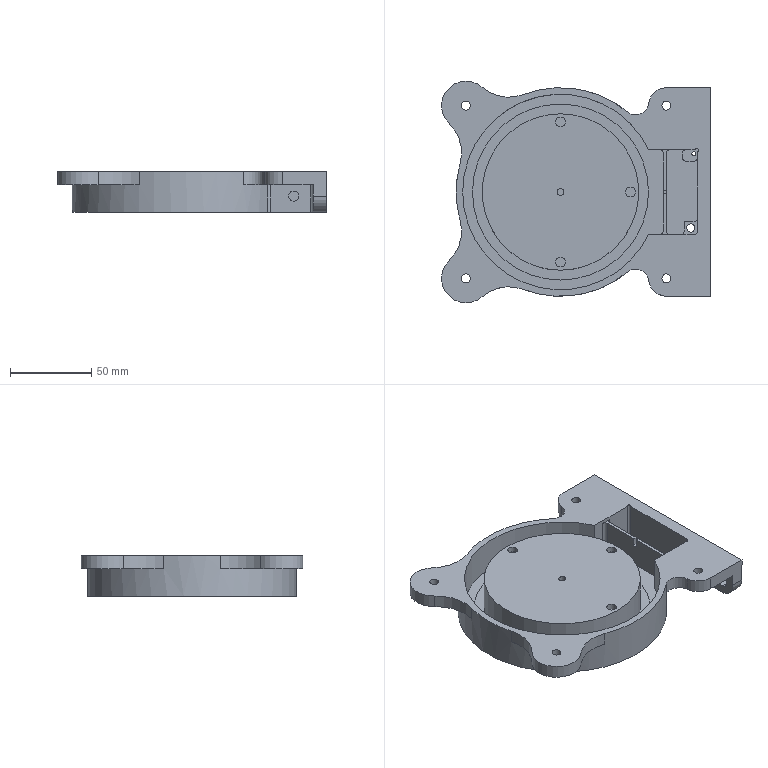NC program | NX | posted with a generic post | part box 165 x 136 x 25 mm
Lines 3306 to 5148 of 5148, first 1627 of 1827 lines:
(CAVITY_MILL_COPY_COPY , TOOL : D4)
N6580 T04 M6
N6582 G54
N6584 G17 G0 G90 X13.936 Y-32.8 S9500 M3
N6586 G43 Z30. H4
N6588 Z0.605
N6590 G94 G1 Z-0.395 F1000.
N6592 X13.763 Y-32.5
N6594 G3 X12.897 Y-32. R1.
N6596 G1 X10. F1500.
N6598 Y-34.897
N6600 G3 X10.5 Y-35.763 R1.
N6602 G1 X10.8 Y-35.936
N6604 Z0.605
N6606 G0 Z30.
N6608 X13.936 Y-32.8
N6610 Z0.209
N6612 G1 Z-0.791 F1000.
N6614 X13.763 Y-32.5
N6616 G3 X12.897 Y-32. R1.
N6618 G1 X10. F1500.
N6620 Y-34.897
N6622 G3 X10.5 Y-35.763 R1.
N6624 G1 X10.8 Y-35.936
N6626 Z0.209
N6628 G0 X13.936 Y-32.8 Z-0.186
N6630 G1 Z-1.186 F1000.
N6632 X13.763 Y-32.5
N6634 G3 X12.897 Y-32. R1.
N6636 G1 X10. F1500.
N6638 Y-34.897
N6640 G3 X10.5 Y-35.763 R1.
N6642 G1 X10.8 Y-35.936
N6644 Z-0.186
N6646 G0 X13.936 Y-32.8 Z-0.581
N6648 G1 Z-1.581 F1000.
N6650 X13.763 Y-32.5
N6652 G3 X12.897 Y-32. R1.
N6654 G1 X10. F1500.
N6656 Y-34.897
N6658 G3 X10.5 Y-35.763 R1.
N6660 G1 X10.8 Y-35.936
N6662 Z-0.581
N6664 G0 X13.936 Y-32.8 Z-0.977
N6666 G1 Z-1.977 F1000.
N6668 X13.763 Y-32.5
N6670 G3 X12.897 Y-32. R1.
N6672 G1 X10. F1500.
N6674 Y-34.897
N6676 G3 X10.5 Y-35.763 R1.
N6678 G1 X10.8 Y-35.936
N6680 Z-0.977
N6682 G0 X13.936 Y-32.8 Z-1.372
N6684 G1 Z-2.372 F1000.
N6686 X13.763 Y-32.5
N6688 G3 X12.897 Y-32. R1.
N6690 G1 X10. F1500.
N6692 Y-34.897
N6694 G3 X10.5 Y-35.763 R1.
N6696 G1 X10.8 Y-35.936
N6698 Z-1.372
N6700 G0 X13.936 Y-32.8 Z-1.767
N6702 G1 Z-2.767 F1000.
N6704 X13.763 Y-32.5
N6706 G3 X12.897 Y-32. R1.
N6708 G1 X10. F1500.
N6710 Y-34.897
N6712 G3 X10.5 Y-35.763 R1.
N6714 G1 X10.8 Y-35.936
N6716 Z-1.767
N6718 G0 X13.936 Y-32.8 Z-2.163
N6720 G1 Z-3.163 F1000.
N6722 X13.763 Y-32.5
N6724 G3 X12.897 Y-32. R1.
N6726 G1 X10. F1500.
N6728 Y-34.897
N6730 G3 X10.5 Y-35.763 R1.
N6732 G1 X10.8 Y-35.936
N6734 Z-2.163
N6736 G0 X13.936 Y-32.8 Z-2.558
N6738 G1 Z-3.558 F1000.
N6740 X13.763 Y-32.5
N6742 G3 X12.897 Y-32. R1.
N6744 G1 X10. F1500.
N6746 Y-34.897
N6748 G3 X10.5 Y-35.763 R1.
N6750 G1 X10.8 Y-35.936
N6752 Z-2.558
N6754 G0 X13.936 Y-32.8 Z-2.953
N6756 G1 Z-3.953 F1000.
N6758 X13.763 Y-32.5
N6760 G3 X12.897 Y-32. R1.
N6762 G1 X10. F1500.
N6764 Y-34.897
N6766 G3 X10.5 Y-35.763 R1.
N6768 G1 X10.8 Y-35.936
N6770 Z-2.953
N6772 G0 X13.936 Y-32.8 Z-3.349
N6774 G1 Z-4.349 F1000.
N6776 X13.763 Y-32.5
N6778 G3 X12.897 Y-32. R1.
N6780 G1 X10. F1500.
N6782 Y-34.897
N6784 G3 X10.5 Y-35.763 R1.
N6786 G1 X10.8 Y-35.936
N6788 Z-3.349
N6790 G0 X13.936 Y-32.8 Z-3.744
N6792 G1 Z-4.744 F1000.
N6794 X13.763 Y-32.5
N6796 G3 X12.897 Y-32. R1.
N6798 G1 X10. F1500.
N6800 Y-34.897
N6802 G3 X10.5 Y-35.763 R1.
N6804 G1 X10.8 Y-35.936
N6806 Z-3.744
N6808 G0 X13.936 Y-32.8 Z-4.14
N6810 G1 Z-5.14 F1000.
N6812 X13.763 Y-32.5
N6814 G3 X12.897 Y-32. R1.
N6816 G1 X10. F1500.
N6818 Y-34.897
N6820 G3 X10.5 Y-35.763 R1.
N6822 G1 X10.8 Y-35.936
N6824 Z-4.14
N6826 G0 X13.936 Y-32.8 Z-4.535
N6828 G1 Z-5.535 F1000.
N6830 X13.763 Y-32.5
N6832 G3 X12.897 Y-32. R1.
N6834 G1 X10. F1500.
N6836 Y-34.897
N6838 G3 X10.5 Y-35.763 R1.
N6840 G1 X10.8 Y-35.936
N6842 Z-4.535
N6844 G0 X13.936 Y-32.8 Z-4.93
N6846 G1 Z-5.93 F1000.
N6848 X13.763 Y-32.5
N6850 G3 X12.897 Y-32. R1.
N6852 G1 X10. F1500.
N6854 Y-34.897
N6856 G3 X10.5 Y-35.763 R1.
N6858 G1 X10.8 Y-35.936
N6860 Z-4.93
N6862 G0 X13.936 Y-32.8 Z-5.326
N6864 G1 Z-6.326 F1000.
N6866 X13.763 Y-32.5
N6868 G3 X12.897 Y-32. R1.
N6870 G1 X10. F1500.
N6872 Y-34.897
N6874 G3 X10.5 Y-35.763 R1.
N6876 G1 X10.8 Y-35.936
N6878 Z-5.326
N6880 G0 X13.936 Y-32.8 Z-5.721
N6882 G1 Z-6.721 F1000.
N6884 X13.763 Y-32.5
N6886 G3 X12.897 Y-32. R1.
N6888 G1 X10. F1500.
N6890 Y-34.897
N6892 G3 X10.5 Y-35.763 R1.
N6894 G1 X10.8 Y-35.936
N6896 Z-5.721
N6898 G0 X13.936 Y-32.8 Z-6.116
N6900 G1 Z-7.116 F1000.
N6902 X13.763 Y-32.5
N6904 G3 X12.897 Y-32. R1.
N6906 G1 X10. F1500.
N6908 Y-34.897
N6910 G3 X10.5 Y-35.763 R1.
N6912 G1 X10.8 Y-35.936
N6914 Z-6.116
N6916 G0 X13.936 Y-32.8 Z-6.512
N6918 G1 Z-7.512 F1000.
N6920 X13.763 Y-32.5
N6922 G3 X12.897 Y-32. R1.
N6924 G1 X10. F1500.
N6926 Y-34.897
N6928 G3 X10.5 Y-35.763 R1.
N6930 G1 X10.8 Y-35.936
N6932 Z-6.512
N6934 G0 X13.936 Y-32.8 Z-6.907
N6936 G1 Z-7.907 F1000.
N6938 X13.763 Y-32.5
N6940 G3 X12.897 Y-32. R1.
N6942 G1 X10. F1500.
N6944 Y-34.897
N6946 G3 X10.5 Y-35.763 R1.
N6948 G1 X10.8 Y-35.936
N6950 Z-6.907
N6952 G0 X13.936 Y-32.8 Z-7.302
N6954 G1 Z-8.302 F1000.
N6956 X13.763 Y-32.5
N6958 G3 X12.897 Y-32. R1.
N6960 G1 X10. F1500.
N6962 Y-34.897
N6964 G3 X10.5 Y-35.763 R1.
N6966 G1 X10.8 Y-35.936
N6968 Z-7.302
N6970 G0 X13.936 Y-32.8 Z-7.698
N6972 G1 Z-8.698 F1000.
N6974 X13.763 Y-32.5
N6976 G3 X12.897 Y-32. R1.
N6978 G1 X10. F1500.
N6980 Y-34.897
N6982 G3 X10.5 Y-35.763 R1.
N6984 G1 X10.8 Y-35.936
N6986 Z-7.698
N6988 G0 X13.936 Y-32.8 Z-8.093
N6990 G1 Z-9.093 F1000.
N6992 X13.763 Y-32.5
N6994 G3 X12.897 Y-32. R1.
N6996 G1 X10. F1500.
N6998 Y-34.897
N7000 G3 X10.5 Y-35.763 R1.
N7002 G1 X10.8 Y-35.936
N7004 Z-8.093
N7006 G0 X13.936 Y-32.8 Z-8.488
N7008 G1 Z-9.488 F1000.
N7010 X13.763 Y-32.5
N7012 G3 X12.897 Y-32. R1.
N7014 G1 X10. F1500.
N7016 Y-34.897
N7018 G3 X10.5 Y-35.763 R1.
N7020 G1 X10.8 Y-35.936
N7022 Z-8.488
N7024 G0 X13.936 Y-32.8 Z-8.884
N7026 G1 Z-9.884 F1000.
N7028 X13.763 Y-32.5
N7030 G3 X12.897 Y-32. R1.
N7032 G1 X10. F1500.
N7034 Y-34.897
N7036 G3 X10.5 Y-35.763 R1.
N7038 G1 X10.8 Y-35.936
N7040 Z-8.884
N7042 G0 X13.936 Y-32.8 Z-9.279
N7044 G1 Z-10.279 F1000.
N7046 X13.763 Y-32.5
N7048 G3 X12.897 Y-32. R1.
N7050 G1 X10. F1500.
N7052 Y-34.897
N7054 G3 X10.5 Y-35.763 R1.
N7056 G1 X10.8 Y-35.936
N7058 Z-9.279
N7060 G0 X13.936 Y-32.8 Z-9.674
N7062 G1 Z-10.674 F1000.
N7064 X13.763 Y-32.5
N7066 G3 X12.897 Y-32. R1.
N7068 G1 X10. F1500.
N7070 Y-34.897
N7072 G3 X10.5 Y-35.763 R1.
N7074 G1 X10.8 Y-35.936
N7076 Z-9.674
N7078 G0 X13.936 Y-32.8 Z-10.07
N7080 G1 Z-11.07 F1000.
N7082 X13.763 Y-32.5
N7084 G3 X12.897 Y-32. R1.
N7086 G1 X10. F1500.
N7088 Y-34.897
N7090 G3 X10.5 Y-35.763 R1.
N7092 G1 X10.8 Y-35.936
N7094 Z-10.07
N7096 G0 X13.936 Y-32.8 Z-10.465
N7098 G1 Z-11.465 F1000.
N7100 X13.763 Y-32.5
N7102 G3 X12.897 Y-32. R1.
N7104 G1 X10. F1500.
N7106 Y-34.897
N7108 G3 X10.5 Y-35.763 R1.
N7110 G1 X10.8 Y-35.936
N7112 Z-10.465
N7114 G0 X13.936 Y-32.8 Z-10.86
N7116 G1 Z-11.86 F1000.
N7118 X13.763 Y-32.5
N7120 G3 X12.897 Y-32. R1.
N7122 G1 X10. F1500.
N7124 Y-34.897
N7126 G3 X10.5 Y-35.763 R1.
N7128 G1 X10.8 Y-35.936
N7130 Z-10.86
N7132 G0 X13.936 Y-32.8 Z-11.256
N7134 G1 Z-12.256 F1000.
N7136 X13.763 Y-32.5
N7138 G3 X12.897 Y-32. R1.
N7140 G1 X10. F1500.
N7142 Y-34.897
N7144 G3 X10.5 Y-35.763 R1.
N7146 G1 X10.8 Y-35.936
N7148 Z-11.256
N7150 G0 X13.936 Y-32.8 Z-11.651
N7152 G1 Z-12.651 F1000.
N7154 X13.763 Y-32.5
N7156 G3 X12.897 Y-32. R1.
N7158 G1 X10. F1500.
N7160 Y-34.897
N7162 G3 X10.5 Y-35.763 R1.
N7164 G1 X10.8 Y-35.936
N7166 Z-11.651
N7168 G0 X13.936 Y-32.8 Z-12.047
N7170 G1 Z-13.047 F1000.
N7172 X13.763 Y-32.5
N7174 G3 X12.897 Y-32. R1.
N7176 G1 X10. F1500.
N7178 Y-34.897
N7180 G3 X10.5 Y-35.763 R1.
N7182 G1 X10.8 Y-35.936
N7184 Z-12.047
N7186 G0 X13.936 Y-32.8 Z-12.442
N7188 G1 Z-13.442 F1000.
N7190 X13.763 Y-32.5
N7192 G3 X12.897 Y-32. R1.
N7194 G1 X10. F1500.
N7196 Y-34.897
N7198 G3 X10.5 Y-35.763 R1.
N7200 G1 X10.8 Y-35.936
N7202 Z-12.442
N7204 G0 X13.936 Y-32.8 Z-12.837
N7206 G1 Z-13.837 F1000.
N7208 X13.763 Y-32.5
N7210 G3 X12.897 Y-32. R1.
N7212 G1 X10. F1500.
N7214 Y-34.897
N7216 G3 X10.5 Y-35.763 R1.
N7218 G1 X10.8 Y-35.936
N7220 Z-12.837
N7222 G0 X13.936 Y-32.8 Z-13.233
N7224 G1 Z-14.233 F1000.
N7226 X13.763 Y-32.5
N7228 G3 X12.897 Y-32. R1.
N7230 G1 X10. F1500.
N7232 Y-34.897
N7234 G3 X10.5 Y-35.763 R1.
N7236 G1 X10.8 Y-35.936
N7238 Z-13.233
N7240 G0 X13.936 Y-32.8 Z-13.628
N7242 G1 Z-14.628 F1000.
N7244 X13.763 Y-32.5
N7246 G3 X12.897 Y-32. R1.
N7248 G1 X10. F1500.
N7250 Y-34.897
N7252 G3 X10.5 Y-35.763 R1.
N7254 G1 X10.8 Y-35.936
N7256 Z-13.628
N7258 G0 X13.936 Y-32.8 Z-14.023
N7260 G1 Z-15.023 F1000.
N7262 X13.763 Y-32.5
N7264 G3 X12.897 Y-32. R1.
N7266 G1 X10. F1500.
N7268 Y-34.897
N7270 G3 X10.5 Y-35.763 R1.
N7272 G1 X10.8 Y-35.936
N7274 Z-14.023
N7276 G0 X13.936 Y-32.8 Z-14.419
N7278 G1 Z-15.419 F1000.
N7280 X13.763 Y-32.5
N7282 G3 X12.897 Y-32. R1.
N7284 G1 X10. F1500.
N7286 Y-34.897
N7288 G3 X10.5 Y-35.763 R1.
N7290 G1 X10.8 Y-35.936
N7292 Z-14.419
N7294 G0 X13.936 Y-32.8 Z-14.814
N7296 G1 Z-15.814 F1000.
N7298 X13.763 Y-32.5
N7300 G3 X12.897 Y-32. R1.
N7302 G1 X10. F1500.
N7304 Y-34.897
N7306 G3 X10.5 Y-35.763 R1.
N7308 G1 X10.8 Y-35.936
N7310 Z-14.814
N7312 G0 X13.936 Y-32.8 Z-15.209
N7314 G1 Z-16.209 F1000.
N7316 X13.763 Y-32.5
N7318 G3 X12.897 Y-32. R1.
N7320 G1 X10. F1500.
N7322 Y-34.897
N7324 G3 X10.5 Y-35.763 R1.
N7326 G1 X10.8 Y-35.936
N7328 Z-15.209
N7330 G0 X13.936 Y-32.8 Z-15.605
N7332 G1 Z-16.605 F1000.
N7334 X13.763 Y-32.5
N7336 G3 X12.897 Y-32. R1.
N7338 G1 X10. F1500.
N7340 Y-34.897
N7342 G3 X10.5 Y-35.763 R1.
N7344 G1 X10.8 Y-35.936
N7346 Z-15.605
N7348 G0 X13.936 Y-32.8 Z-16.
N7350 G1 Z-17. F1000.
N7352 X13.763 Y-32.5
N7354 G3 X12.897 Y-32. R1.
N7356 G1 X10. F1500.
N7358 Y-34.897
N7360 G3 X10.5 Y-35.763 R1.
N7362 G1 X10.8 Y-35.936
N7364 Z-16.
N7366 G0 Z30.
N7368 X34.916 Y-34.694
N7370 Z0.605
N7372 G1 Z-0.395 F1000.
N7374 X35.083 Y-34.401
N7376 G3 X35.076 Y-33.401 R1.
N7378 G2 X34.277 Y-32. R66. F1500.
N7380 G1 X32.639
N7382 G3 X31.773 Y-32.5 R1.
N7384 G1 X31.599 Y-32.8
N7386 Z0.605
N7388 G0 Z30.
N7390 X34.916 Y-34.694
N7392 Z0.209
N7394 G1 Z-0.791 F1000.
N7396 X35.083 Y-34.401
N7398 G3 X35.076 Y-33.401 R1.
N7400 G2 X34.277 Y-32. R66. F1500.
N7402 G1 X32.639
N7404 G3 X31.773 Y-32.5 R1.
N7406 G1 X31.599 Y-32.8
N7408 Z0.209
N7410 G0 X34.916 Y-34.694 Z-0.186
N7412 G1 Z-1.186 F1000.
N7414 X35.083 Y-34.401
N7416 G3 X35.076 Y-33.401 R1.
N7418 G2 X34.277 Y-32. R66. F1500.
N7420 G1 X32.639
N7422 G3 X31.773 Y-32.5 R1.
N7424 G1 X31.599 Y-32.8
N7426 Z-0.186
N7428 G0 X34.916 Y-34.694 Z-0.581
N7430 G1 Z-1.581 F1000.
N7432 X35.083 Y-34.401
N7434 G3 X35.076 Y-33.401 R1.
N7436 G2 X34.277 Y-32. R66. F1500.
N7438 G1 X32.639
N7440 G3 X31.773 Y-32.5 R1.
N7442 G1 X31.599 Y-32.8
N7444 Z-0.581
N7446 G0 X34.916 Y-34.694 Z-0.977
N7448 G1 Z-1.977 F1000.
N7450 X35.083 Y-34.401
N7452 G3 X35.076 Y-33.401 R1.
N7454 G2 X34.277 Y-32. R66. F1500.
N7456 G1 X32.639
N7458 G3 X31.773 Y-32.5 R1.
N7460 G1 X31.599 Y-32.8
N7462 Z-0.977
N7464 G0 X34.916 Y-34.694 Z-1.372
N7466 G1 Z-2.372 F1000.
N7468 X35.083 Y-34.401
N7470 G3 X35.076 Y-33.401 R1.
N7472 G2 X34.277 Y-32. R66. F1500.
N7474 G1 X32.639
N7476 G3 X31.773 Y-32.5 R1.
N7478 G1 X31.599 Y-32.8
N7480 Z-1.372
N7482 G0 X34.916 Y-34.694 Z-1.767
N7484 G1 Z-2.767 F1000.
N7486 X35.083 Y-34.401
N7488 G3 X35.076 Y-33.401 R1.
N7490 G2 X34.277 Y-32. R66. F1500.
N7492 G1 X32.639
N7494 G3 X31.773 Y-32.5 R1.
N7496 G1 X31.599 Y-32.8
N7498 Z-1.767
N7500 G0 X34.916 Y-34.694 Z-2.163
N7502 G1 Z-3.163 F1000.
N7504 X35.083 Y-34.401
N7506 G3 X35.076 Y-33.401 R1.
N7508 G2 X34.277 Y-32. R66. F1500.
N7510 G1 X32.639
N7512 G3 X31.773 Y-32.5 R1.
N7514 G1 X31.599 Y-32.8
N7516 Z-2.163
N7518 G0 X34.916 Y-34.694 Z-2.558
N7520 G1 Z-3.558 F1000.
N7522 X35.083 Y-34.401
N7524 G3 X35.076 Y-33.401 R1.
N7526 G2 X34.277 Y-32. R66. F1500.
N7528 G1 X32.639
N7530 G3 X31.773 Y-32.5 R1.
N7532 G1 X31.599 Y-32.8
N7534 Z-2.558
N7536 G0 X34.916 Y-34.694 Z-2.953
N7538 G1 Z-3.953 F1000.
N7540 X35.083 Y-34.401
N7542 G3 X35.076 Y-33.401 R1.
N7544 G2 X34.277 Y-32. R66. F1500.
N7546 G1 X32.639
N7548 G3 X31.773 Y-32.5 R1.
N7550 G1 X31.599 Y-32.8
N7552 Z-2.953
N7554 G0 X34.916 Y-34.694 Z-3.349
N7556 G1 Z-4.349 F1000.
N7558 X35.083 Y-34.401
N7560 G3 X35.076 Y-33.401 R1.
N7562 G2 X34.277 Y-32. R66. F1500.
N7564 G1 X32.639
N7566 G3 X31.773 Y-32.5 R1.
N7568 G1 X31.599 Y-32.8
N7570 Z-3.349
N7572 G0 X34.916 Y-34.694 Z-3.744
N7574 G1 Z-4.744 F1000.
N7576 X35.083 Y-34.401
N7578 G3 X35.076 Y-33.401 R1.
N7580 G2 X34.277 Y-32. R66. F1500.
N7582 G1 X32.639
N7584 G3 X31.773 Y-32.5 R1.
N7586 G1 X31.599 Y-32.8
N7588 Z-3.744
N7590 G0 X34.916 Y-34.694 Z-4.14
N7592 G1 Z-5.14 F1000.
N7594 X35.083 Y-34.401
N7596 G3 X35.076 Y-33.401 R1.
N7598 G2 X34.277 Y-32. R66. F1500.
N7600 G1 X32.639
N7602 G3 X31.773 Y-32.5 R1.
N7604 G1 X31.599 Y-32.8
N7606 Z-4.14
N7608 G0 X34.916 Y-34.694 Z-4.535
N7610 G1 Z-5.535 F1000.
N7612 X35.083 Y-34.401
N7614 G3 X35.076 Y-33.401 R1.
N7616 G2 X34.277 Y-32. R66. F1500.
N7618 G1 X32.639
N7620 G3 X31.773 Y-32.5 R1.
N7622 G1 X31.599 Y-32.8
N7624 Z-4.535
N7626 G0 X34.916 Y-34.694 Z-4.93
N7628 G1 Z-5.93 F1000.
N7630 X35.083 Y-34.401
N7632 G3 X35.076 Y-33.401 R1.
N7634 G2 X34.277 Y-32. R66. F1500.
N7636 G1 X32.639
N7638 G3 X31.773 Y-32.5 R1.
N7640 G1 X31.599 Y-32.8
N7642 Z-4.93
N7644 G0 X34.916 Y-34.694 Z-5.326
N7646 G1 Z-6.326 F1000.
N7648 X35.083 Y-34.401
N7650 G3 X35.076 Y-33.401 R1.
N7652 G2 X34.277 Y-32. R66. F1500.
N7654 G1 X32.639
N7656 G3 X31.773 Y-32.5 R1.
N7658 G1 X31.599 Y-32.8
N7660 Z-5.326
N7662 G0 X34.916 Y-34.694 Z-5.721
N7664 G1 Z-6.721 F1000.
N7666 X35.083 Y-34.401
N7668 G3 X35.076 Y-33.401 R1.
N7670 G2 X34.277 Y-32. R66. F1500.
N7672 G1 X32.639
N7674 G3 X31.773 Y-32.5 R1.
N7676 G1 X31.599 Y-32.8
N7678 Z-5.721
N7680 G0 X34.916 Y-34.694 Z-6.116
N7682 G1 Z-7.116 F1000.
N7684 X35.083 Y-34.401
N7686 G3 X35.076 Y-33.401 R1.
N7688 G2 X34.277 Y-32. R66. F1500.
N7690 G1 X32.639
N7692 G3 X31.773 Y-32.5 R1.
N7694 G1 X31.599 Y-32.8
N7696 Z-6.116
N7698 G0 X34.916 Y-34.694 Z-6.512
N7700 G1 Z-7.512 F1000.
N7702 X35.083 Y-34.401
N7704 G3 X35.076 Y-33.401 R1.
N7706 G2 X34.277 Y-32. R66. F1500.
N7708 G1 X32.639
N7710 G3 X31.773 Y-32.5 R1.
N7712 G1 X31.599 Y-32.8
N7714 Z-6.512
N7716 G0 X34.916 Y-34.694 Z-6.907
N7718 G1 Z-7.907 F1000.
N7720 X35.083 Y-34.401
N7722 G3 X35.076 Y-33.401 R1.
N7724 G2 X34.277 Y-32. R66. F1500.
N7726 G1 X32.639
N7728 G3 X31.773 Y-32.5 R1.
N7730 G1 X31.599 Y-32.8
N7732 Z-6.907
N7734 G0 X34.916 Y-34.694 Z-7.302
N7736 G1 Z-8.302 F1000.
N7738 X35.083 Y-34.401
N7740 G3 X35.076 Y-33.401 R1.
N7742 G2 X34.277 Y-32. R66. F1500.
N7744 G1 X32.639
N7746 G3 X31.773 Y-32.5 R1.
N7748 G1 X31.599 Y-32.8
N7750 Z-7.302
N7752 G0 X34.916 Y-34.694 Z-7.698
N7754 G1 Z-8.698 F1000.
N7756 X35.083 Y-34.401
N7758 G3 X35.076 Y-33.401 R1.
N7760 G2 X34.277 Y-32. R66. F1500.
N7762 G1 X32.639
N7764 G3 X31.773 Y-32.5 R1.
N7766 G1 X31.599 Y-32.8
N7768 Z-7.698
N7770 G0 X34.916 Y-34.694 Z-8.093
N7772 G1 Z-9.093 F1000.
N7774 X35.083 Y-34.401
N7776 G3 X35.076 Y-33.401 R1.
N7778 G2 X34.277 Y-32. R66. F1500.
N7780 G1 X32.639
N7782 G3 X31.773 Y-32.5 R1.
N7784 G1 X31.599 Y-32.8
N7786 Z-8.093
N7788 G0 X34.916 Y-34.694 Z-8.488
N7790 G1 Z-9.488 F1000.
N7792 X35.083 Y-34.401
N7794 G3 X35.076 Y-33.401 R1.
N7796 G2 X34.277 Y-32. R66. F1500.
N7798 G1 X32.639
N7800 G3 X31.773 Y-32.5 R1.
N7802 G1 X31.599 Y-32.8
N7804 Z-8.488
N7806 G0 X34.916 Y-34.694 Z-8.884
N7808 G1 Z-9.884 F1000.
N7810 X35.083 Y-34.401
N7812 G3 X35.076 Y-33.401 R1.
N7814 G2 X34.277 Y-32. R66. F1500.
N7816 G1 X32.639
N7818 G3 X31.773 Y-32.5 R1.
N7820 G1 X31.599 Y-32.8
N7822 Z-8.884
N7824 G0 X34.916 Y-34.694 Z-9.279
N7826 G1 Z-10.279 F1000.
N7828 X35.083 Y-34.401
N7830 G3 X35.076 Y-33.401 R1.
N7832 G2 X34.277 Y-32. R66. F1500.
N7834 G1 X32.639
N7836 G3 X31.773 Y-32.5 R1.
N7838 G1 X31.599 Y-32.8
N7840 Z-9.279
N7842 G0 X34.916 Y-34.694 Z-9.674
N7844 G1 Z-10.674 F1000.
N7846 X35.083 Y-34.401
N7848 G3 X35.076 Y-33.401 R1.
N7850 G2 X34.277 Y-32. R66. F1500.
N7852 G1 X32.639
N7854 G3 X31.773 Y-32.5 R1.
N7856 G1 X31.599 Y-32.8
N7858 Z-9.674
N7860 G0 X34.916 Y-34.694 Z-10.07
N7862 G1 Z-11.07 F1000.
N7864 X35.083 Y-34.401
N7866 G3 X35.076 Y-33.401 R1.
N7868 G2 X34.277 Y-32. R66. F1500.
N7870 G1 X32.639
N7872 G3 X31.773 Y-32.5 R1.
N7874 G1 X31.599 Y-32.8
N7876 Z-10.07
N7878 G0 X34.916 Y-34.694 Z-10.465
N7880 G1 Z-11.465 F1000.
N7882 X35.083 Y-34.401
N7884 G3 X35.076 Y-33.401 R1.
N7886 G2 X34.277 Y-32. R66. F1500.
N7888 G1 X32.639
N7890 G3 X31.773 Y-32.5 R1.
N7892 G1 X31.599 Y-32.8
N7894 Z-10.465
N7896 G0 X34.916 Y-34.694 Z-10.86
N7898 G1 Z-11.86 F1000.
N7900 X35.083 Y-34.401
N7902 G3 X35.076 Y-33.401 R1.
N7904 G2 X34.277 Y-32. R66. F1500.
N7906 G1 X32.639
N7908 G3 X31.773 Y-32.5 R1.
N7910 G1 X31.599 Y-32.8
N7912 Z-10.86
N7914 G0 X34.916 Y-34.694 Z-11.256
N7916 G1 Z-12.256 F1000.
N7918 X35.083 Y-34.401
N7920 G3 X35.076 Y-33.401 R1.
N7922 G2 X34.277 Y-32. R66. F1500.
N7924 G1 X32.639
N7926 G3 X31.773 Y-32.5 R1.
N7928 G1 X31.599 Y-32.8
N7930 Z-11.256
N7932 G0 X34.916 Y-34.694 Z-11.651
N7934 G1 Z-12.651 F1000.
N7936 X35.083 Y-34.401
N7938 G3 X35.076 Y-33.401 R1.
N7940 G2 X34.277 Y-32. R66. F1500.
N7942 G1 X32.639
N7944 G3 X31.773 Y-32.5 R1.
N7946 G1 X31.599 Y-32.8
N7948 Z-11.651
N7950 G0 X34.916 Y-34.694 Z-12.047
N7952 G1 Z-13.047 F1000.
N7954 X35.083 Y-34.401
N7956 G3 X35.076 Y-33.401 R1.
N7958 G2 X34.277 Y-32. R66. F1500.
N7960 G1 X32.639
N7962 G3 X31.773 Y-32.5 R1.
N7964 G1 X31.599 Y-32.8
N7966 Z-12.047
N7968 G0 X34.916 Y-34.694 Z-12.442
N7970 G1 Z-13.442 F1000.
N7972 X35.083 Y-34.401
N7974 G3 X35.076 Y-33.401 R1.
N7976 G2 X34.277 Y-32. R66. F1500.
N7978 G1 X32.639
N7980 G3 X31.773 Y-32.5 R1.
N7982 G1 X31.599 Y-32.8
N7984 Z-12.442
N7986 G0 X34.916 Y-34.694 Z-12.837
N7988 G1 Z-13.837 F1000.
N7990 X35.083 Y-34.401
N7992 G3 X35.076 Y-33.401 R1.
N7994 G2 X34.277 Y-32. R66. F1500.
N7996 G1 X32.639
N7998 G3 X31.773 Y-32.5 R1.
N8000 G1 X31.599 Y-32.8
N8002 Z-12.837
N8004 G0 X34.916 Y-34.694 Z-13.233
N8006 G1 Z-14.233 F1000.
N8008 X35.083 Y-34.401
N8010 G3 X35.076 Y-33.401 R1.
N8012 G2 X34.277 Y-32. R66. F1500.
N8014 G1 X32.639
N8016 G3 X31.773 Y-32.5 R1.
N8018 G1 X31.599 Y-32.8
N8020 Z-13.233
N8022 G0 X34.916 Y-34.694 Z-13.628
N8024 G1 Z-14.628 F1000.
N8026 X35.083 Y-34.401
N8028 G3 X35.076 Y-33.401 R1.
N8030 G2 X34.277 Y-32. R66. F1500.
N8032 G1 X32.639
N8034 G3 X31.773 Y-32.5 R1.
N8036 G1 X31.599 Y-32.8
N8038 Z-13.628
N8040 G0 X34.916 Y-34.694 Z-14.023
N8042 G1 Z-15.023 F1000.
N8044 X35.083 Y-34.401
N8046 G3 X35.076 Y-33.401 R1.
N8048 G2 X34.277 Y-32. R66. F1500.
N8050 G1 X32.639
N8052 G3 X31.773 Y-32.5 R1.
N8054 G1 X31.599 Y-32.8
N8056 Z-14.023
N8058 G0 X34.916 Y-34.694 Z-14.419
N8060 G1 Z-15.419 F1000.
N8062 X35.083 Y-34.401
N8064 G3 X35.076 Y-33.401 R1.
N8066 G2 X34.277 Y-32. R66. F1500.
N8068 G1 X32.639
N8070 G3 X31.773 Y-32.5 R1.
N8072 G1 X31.599 Y-32.8
N8074 Z-14.419
N8076 G0 X34.916 Y-34.694 Z-14.814
N8078 G1 Z-15.814 F1000.
N8080 X35.083 Y-34.401
N8082 G3 X35.076 Y-33.401 R1.
N8084 G2 X34.277 Y-32. R66. F1500.
N8086 G1 X32.639
N8088 G3 X31.773 Y-32.5 R1.
N8090 G1 X31.599 Y-32.8
N8092 Z-14.814
N8094 G0 X34.916 Y-34.694 Z-15.209
N8096 G1 Z-16.209 F1000.
N8098 X35.083 Y-34.401
N8100 G3 X35.076 Y-33.401 R1.
N8102 G2 X34.277 Y-32. R66. F1500.
N8104 G1 X32.639
N8106 G3 X31.773 Y-32.5 R1.
N8108 G1 X31.599 Y-32.8
N8110 Z-15.209
N8112 G0 X34.916 Y-34.694 Z-15.605
N8114 G1 Z-16.605 F1000.
N8116 X35.083 Y-34.401
N8118 G3 X35.076 Y-33.401 R1.
N8120 G2 X34.277 Y-32. R66. F1500.
N8122 G1 X32.639
N8124 G3 X31.773 Y-32.5 R1.
N8126 G1 X31.599 Y-32.8
N8128 Z-15.605
N8130 G0 X34.916 Y-34.694 Z-16.
N8132 G1 Z-17. F1000.
N8134 X35.083 Y-34.401
N8136 G3 X35.076 Y-33.401 R1.
N8138 G2 X34.277 Y-32. R66. F1500.
N8140 G1 X32.639
N8142 G3 X31.773 Y-32.5 R1.
N8144 G1 X31.599 Y-32.8
N8146 Z-16.
N8148 G0 Z30.
N8150 Y32.8
N8152 Z0.605
N8154 G1 Z-0.395 F1000.
N8156 X31.773 Y32.5
N8158 G3 X32.639 Y32. R1.
N8160 G1 X34.277 F1500.
N8162 G2 X35.076 Y33.401 R66.
N8164 G3 X35.083 Y34.401 R1.
N8166 G1 X34.916 Y34.694
N8168 Z0.605
N8170 G0 Z30.
N8172 X31.599 Y32.8
N8174 Z0.209
N8176 G1 Z-0.791 F1000.
N8178 X31.773 Y32.5
N8180 G3 X32.639 Y32. R1.
N8182 G1 X34.277 F1500.
N8184 G2 X35.076 Y33.401 R66.
N8186 G3 X35.083 Y34.401 R1.
N8188 G1 X34.916 Y34.694
N8190 Z0.209
N8192 G0 X31.599 Y32.8 Z-0.186
N8194 G1 Z-1.186 F1000.
N8196 X31.773 Y32.5
N8198 G3 X32.639 Y32. R1.
N8200 G1 X34.277 F1500.
N8202 G2 X35.076 Y33.401 R66.
N8204 G3 X35.083 Y34.401 R1.
N8206 G1 X34.916 Y34.694
N8208 Z-0.186
N8210 G0 X31.599 Y32.8 Z-0.581
N8212 G1 Z-1.581 F1000.
N8214 X31.773 Y32.5
N8216 G3 X32.639 Y32. R1.
N8218 G1 X34.277 F1500.
N8220 G2 X35.076 Y33.401 R66.
N8222 G3 X35.083 Y34.401 R1.
N8224 G1 X34.916 Y34.694
N8226 Z-0.581
N8228 G0 X31.599 Y32.8 Z-0.977
N8230 G1 Z-1.977 F1000.
N8232 X31.773 Y32.5
N8234 G3 X32.639 Y32. R1.
N8236 G1 X34.277 F1500.
N8238 G2 X35.076 Y33.401 R66.
N8240 G3 X35.083 Y34.401 R1.
N8242 G1 X34.916 Y34.694
N8244 Z-0.977
N8246 G0 X31.599 Y32.8 Z-1.372
N8248 G1 Z-2.372 F1000.
N8250 X31.773 Y32.5
N8252 G3 X32.639 Y32. R1.
N8254 G1 X34.277 F1500.
N8256 G2 X35.076 Y33.401 R66.
N8258 G3 X35.083 Y34.401 R1.
N8260 G1 X34.916 Y34.694
N8262 Z-1.372
N8264 G0 X31.599 Y32.8 Z-1.767
N8266 G1 Z-2.767 F1000.
N8268 X31.773 Y32.5
N8270 G3 X32.639 Y32. R1.
N8272 G1 X34.277 F1500.
N8274 G2 X35.076 Y33.401 R66.
N8276 G3 X35.083 Y34.401 R1.
N8278 G1 X34.916 Y34.694
N8280 Z-1.767
N8282 G0 X31.599 Y32.8 Z-2.163
N8284 G1 Z-3.163 F1000.
N8286 X31.773 Y32.5
N8288 G3 X32.639 Y32. R1.
N8290 G1 X34.277 F1500.
N8292 G2 X35.076 Y33.401 R66.
N8294 G3 X35.083 Y34.401 R1.
N8296 G1 X34.916 Y34.694
N8298 Z-2.163
N8300 G0 X31.599 Y32.8 Z-2.558
N8302 G1 Z-3.558 F1000.
N8304 X31.773 Y32.5
N8306 G3 X32.639 Y32. R1.
N8308 G1 X34.277 F1500.
N8310 G2 X35.076 Y33.401 R66.
N8312 G3 X35.083 Y34.401 R1.
N8314 G1 X34.916 Y34.694
N8316 Z-2.558
N8318 G0 X31.599 Y32.8 Z-2.953
N8320 G1 Z-3.953 F1000.
N8322 X31.773 Y32.5
N8324 G3 X32.639 Y32. R1.
N8326 G1 X34.277 F1500.
N8328 G2 X35.076 Y33.401 R66.
N8330 G3 X35.083 Y34.401 R1.
N8332 G1 X34.916 Y34.695
N8334 Z-2.953
N8336 G0 X31.599 Y32.8 Z-3.349
N8338 G1 Z-4.349 F1000.
N8340 X31.773 Y32.5
N8342 G3 X32.639 Y32. R1.
N8344 G1 X34.277 F1500.
N8346 G2 X35.076 Y33.401 R66.
N8348 G3 X35.083 Y34.401 R1.
N8350 G1 X34.917 Y34.695
N8352 Z-3.349
N8354 G0 X31.599 Y32.8 Z-3.744
N8356 G1 Z-4.744 F1000.
N8358 X31.773 Y32.5
N8360 G3 X32.639 Y32. R1.
N8362 G1 X34.277 F1500.
N8364 G2 X35.076 Y33.401 R66.
N8366 G3 X35.083 Y34.401 R1.
N8368 G1 X34.917 Y34.695
N8370 Z-3.744
N8372 G0 X31.599 Y32.8 Z-4.14
N8374 G1 Z-5.14 F1000.
N8376 X31.772 Y32.5
N8378 G3 X32.639 Y32. R1.
N8380 G1 X34.277 F1500.
N8382 G2 X35.076 Y33.402 R66.
N8384 G3 X35.083 Y34.402 R1.
N8386 G1 X34.917 Y34.695
N8388 Z-4.14
N8390 G0 X31.599 Y32.8 Z-4.535
N8392 G1 Z-5.535 F1000.
N8394 X31.772 Y32.5
N8396 G3 X32.638 Y32. R1.
N8398 G1 X34.277 F1500.
N8400 G2 X35.076 Y33.402 R66.
N8402 G3 X35.083 Y34.402 R1.
N8404 G1 X34.917 Y34.695
N8406 Z-4.535
N8408 G0 X31.599 Y32.8 Z-4.93
N8410 G1 Z-5.93 F1000.
N8412 X31.772 Y32.5
N8414 G3 X32.638 Y32. R1.
N8416 G1 X34.277 F1500.
N8418 G2 X35.076 Y33.402 R66.
N8420 G3 X35.083 Y34.402 R1.
N8422 G1 X34.917 Y34.695
N8424 Z-4.93
N8426 G0 X31.599 Y32.8 Z-5.326
N8428 G1 Z-6.326 F1000.
N8430 X31.772 Y32.5
N8432 G3 X32.638 Y32. R1.
N8434 G1 X34.277 F1500.
N8436 G2 X35.076 Y33.402 R66.
N8438 G3 X35.083 Y34.402 R1.
N8440 G1 X34.917 Y34.695
N8442 Z-5.326
N8444 G0 X31.599 Y32.8 Z-5.721
N8446 G1 Z-6.721 F1000.
N8448 X31.772 Y32.5
N8450 G3 X32.638 Y32. R1.
N8452 G1 X34.277 F1500.
N8454 G2 X35.076 Y33.402 R66.
N8456 G3 X35.083 Y34.402 R1.
N8458 G1 X34.917 Y34.695
N8460 Z-5.721
N8462 G0 X31.599 Y32.8 Z-6.116
N8464 G1 Z-7.116 F1000.
N8466 X31.772 Y32.5
N8468 G3 X32.638 Y32. R1.
N8470 G1 X34.277 F1500.
N8472 G2 X35.076 Y33.402 R66.
N8474 G3 X35.083 Y34.402 R1.
N8476 G1 X34.917 Y34.695
N8478 Z-6.116
N8480 G0 X31.599 Y32.8 Z-6.512
N8482 G1 Z-7.512 F1000.
N8484 X31.772 Y32.5
N8486 G3 X32.638 Y32. R1.
N8488 G1 X34.277 F1500.
N8490 G2 X35.076 Y33.402 R66.
N8492 G3 X35.083 Y34.402 R1.
N8494 G1 X34.917 Y34.695
N8496 Z-6.512
N8498 G0 X31.599 Y32.8 Z-6.907
N8500 G1 Z-7.907 F1000.
N8502 X31.772 Y32.5
N8504 G3 X32.638 Y32. R1.
N8506 G1 X34.277 F1500.
N8508 G2 X35.076 Y33.402 R66.
N8510 G3 X35.083 Y34.402 R1.
N8512 G1 X34.917 Y34.695
N8514 Z-6.907
N8516 G0 X31.599 Y32.8 Z-7.302
N8518 G1 Z-8.302 F1000.
N8520 X31.772 Y32.5
N8522 G3 X32.638 Y32. R1.
N8524 G1 X34.277 F1500.
N8526 G2 X35.076 Y33.401 R66.
N8528 G3 X35.083 Y34.401 R1.
N8530 G1 X34.916 Y34.694
N8532 Z-7.302
N8534 G0 X31.599 Y32.8 Z-7.698
N8536 G1 Z-8.698 F1000.
N8538 X31.772 Y32.5
N8540 G3 X32.638 Y32. R1.
N8542 G1 X34.277 F1500.
N8544 G2 X35.076 Y33.401 R66.
N8546 G3 X35.083 Y34.401 R1.
N8548 G1 X34.916 Y34.694
N8550 Z-7.698
N8552 G0 X31.599 Y32.8 Z-8.093
N8554 G1 Z-9.093 F1000.
N8556 X31.772 Y32.5
N8558 G3 X32.638 Y32. R1.
N8560 G1 X34.277 F1500.
N8562 G2 X35.076 Y33.401 R66.
N8564 G3 X35.083 Y34.401 R1.
N8566 G1 X34.916 Y34.694
N8568 Z-8.093
N8570 G0 X31.599 Y32.8 Z-8.488
N8572 G1 Z-9.488 F1000.
N8574 X31.772 Y32.5
N8576 G3 X32.638 Y32. R1.
N8578 G1 X34.277 F1500.
N8580 G2 X35.076 Y33.401 R66.
N8582 G3 X35.083 Y34.401 R1.
N8584 G1 X34.916 Y34.694
N8586 Z-8.488
N8588 G0 X31.599 Y32.8 Z-8.884
N8590 G1 Z-9.884 F1000.
N8592 X31.772 Y32.5
N8594 G3 X32.638 Y32. R1.
N8596 G1 X34.277 F1500.
N8598 G2 X35.076 Y33.401 R66.
N8600 G3 X35.083 Y34.401 R1.
N8602 G1 X34.916 Y34.694
N8604 Z-8.884
N8606 G0 X31.599 Y32.8 Z-9.279
N8608 G1 Z-10.279 F1000.
N8610 X31.772 Y32.5
N8612 G3 X32.638 Y32. R1.
N8614 G1 X34.277 F1500.
N8616 G2 X35.076 Y33.401 R66.
N8618 G3 X35.083 Y34.401 R1.
N8620 G1 X34.916 Y34.694
N8622 Z-9.279
N8624 G0 X31.599 Y32.8 Z-9.674
N8626 G1 Z-10.674 F1000.
N8628 X31.772 Y32.5
N8630 G3 X32.638 Y32. R1.
N8632 G1 X34.277 F1500.
N8634 G2 X35.076 Y33.401 R66.
N8636 G3 X35.083 Y34.401 R1.
N8638 G1 X34.916 Y34.694
N8640 Z-9.674
N8642 G0 X31.599 Y32.8 Z-10.07
N8644 G1 Z-11.07 F1000.
N8646 X31.772 Y32.5
N8648 G3 X32.638 Y32. R1.
N8650 G1 X34.277 F1500.
N8652 G2 X35.076 Y33.401 R66.
N8654 G3 X35.083 Y34.401 R1.
N8656 G1 X34.916 Y34.694
N8658 Z-10.07
N8660 G0 X31.599 Y32.8 Z-10.465
N8662 G1 Z-11.465 F1000.
N8664 X31.772 Y32.5
N8666 G3 X32.638 Y32. R1.
N8668 G1 X34.277 F1500.
N8670 G2 X35.076 Y33.401 R66.
N8672 G3 X35.083 Y34.401 R1.
N8674 G1 X34.916 Y34.694
N8676 Z-10.465
N8678 G0 X31.599 Y32.8 Z-10.86
N8680 G1 Z-11.86 F1000.
N8682 X31.772 Y32.5
N8684 G3 X32.638 Y32. R1.
N8686 G1 X34.277 F1500.
N8688 G2 X35.076 Y33.401 R66.
N8690 G3 X35.083 Y34.401 R1.
N8692 G1 X34.916 Y34.694
N8694 Z-10.86
N8696 G0 X31.599 Y32.8 Z-11.256
N8698 G1 Z-12.256 F1000.
N8700 X31.772 Y32.5
N8702 G3 X32.638 Y32. R1.
N8704 G1 X34.277 F1500.
N8706 G2 X35.076 Y33.401 R66.
N8708 G3 X35.083 Y34.401 R1.
N8710 G1 X34.916 Y34.694
N8712 Z-11.256
N8714 G0 X31.599 Y32.8 Z-11.651
N8716 G1 Z-12.651 F1000.
N8718 X31.772 Y32.5
N8720 G3 X32.638 Y32. R1.
N8722 G1 X34.277 F1500.
N8724 G2 X35.076 Y33.401 R66.
N8726 G3 X35.083 Y34.401 R1.
N8728 G1 X34.916 Y34.694
N8730 Z-11.651
N8732 G0 X31.599 Y32.8 Z-12.047
N8734 G1 Z-13.047 F1000.
N8736 X31.772 Y32.5
N8738 G3 X32.638 Y32. R1.
N8740 G1 X34.277 F1500.
N8742 G2 X35.076 Y33.401 R66.
N8744 G3 X35.083 Y34.401 R1.
N8746 G1 X34.916 Y34.694
N8748 Z-12.047
N8750 G0 X31.599 Y32.8 Z-12.442
N8752 G1 Z-13.442 F1000.
N8754 X31.772 Y32.5
N8756 G3 X32.638 Y32. R1.
N8758 G1 X34.277 F1500.
N8760 G2 X35.076 Y33.401 R66.
N8762 G3 X35.083 Y34.401 R1.
N8764 G1 X34.916 Y34.694
N8766 Z-12.442
N8768 G0 X31.599 Y32.8 Z-12.837
N8770 G1 Z-13.837 F1000.
N8772 X31.772 Y32.5
N8774 G3 X32.638 Y32. R1.
N8776 G1 X34.277 F1500.
N8778 G2 X35.076 Y33.401 R66.
N8780 G3 X35.083 Y34.401 R1.
N8782 G1 X34.916 Y34.694
N8784 Z-12.837
N8786 G0 X31.599 Y32.8 Z-13.233
N8788 G1 Z-14.233 F1000.
N8790 X31.772 Y32.5
N8792 G3 X32.638 Y32. R1.
N8794 G1 X34.277 F1500.
N8796 G2 X35.076 Y33.401 R66.
N8798 G3 X35.083 Y34.401 R1.
N8800 G1 X34.916 Y34.694
N8802 Z-13.233
N8804 G0 X31.599 Y32.8 Z-13.628
N8806 G1 Z-14.628 F1000.
N8808 X31.772 Y32.5
N8810 G3 X32.638 Y32. R1.
N8812 G1 X34.277 F1500.
N8814 G2 X35.076 Y33.401 R66.
N8816 G3 X35.083 Y34.401 R1.
N8818 G1 X34.916 Y34.695
N8820 Z-13.628
N8822 G0 X31.599 Y32.8 Z-14.023
N8824 G1 Z-15.023 F1000.
N8826 X31.772 Y32.5
N8828 G3 X32.638 Y32. R1.
N8830 G1 X34.277 F1500.
N8832 G2 X35.076 Y33.401 R66.
N8834 G3 X35.083 Y34.401 R1.
N8836 G1 X34.916 Y34.695
N8838 Z-14.023
N8840 G0 X31.599 Y32.8 Z-14.419
N8842 G1 Z-15.419 F1000.
N8844 X31.772 Y32.5
N8846 G3 X32.638 Y32. R1.
N8848 G1 X34.277 F1500.
N8850 G2 X35.076 Y33.401 R66.
N8852 G3 X35.083 Y34.401 R1.
N8854 G1 X34.916 Y34.695
N8856 Z-14.419
N8858 G0 X31.599 Y32.8 Z-14.814
N8860 G1 Z-15.814 F1000.
N8862 X31.772 Y32.5
N8864 G3 X32.638 Y32. R1.
N8866 G1 X34.277 F1500.
N8868 G2 X35.076 Y33.401 R66.
N8870 G3 X35.083 Y34.401 R1.
N8872 G1 X34.916 Y34.695
N8874 Z-14.814
N8876 G0 X31.599 Y32.8 Z-15.209
N8878 G1 Z-16.209 F1000.
N8880 X31.772 Y32.5
N8882 G3 X32.638 Y32. R1.
N8884 G1 X34.277 F1500.
N8886 G2 X35.076 Y33.401 R66.
N8888 G3 X35.083 Y34.401 R1.
N8890 G1 X34.916 Y34.695
N8892 Z-15.209
N8894 G0 X31.599 Y32.8 Z-15.605
N8896 G1 Z-16.605 F1000.
N8898 X31.772 Y32.5
N8900 G3 X32.638 Y32. R1.
N8902 G1 X34.277 F1500.
N8904 G2 X35.076 Y33.401 R66.
N8906 G3 X35.083 Y34.401 R1.
N8908 G1 X34.916 Y34.695
N8910 Z-15.605
N8912 G0 X31.599 Y32.8 Z-16.
N8914 G1 Z-17. F1000.
N8916 X31.772 Y32.5
N8918 G3 X32.638 Y32. R1.
N8920 G1 X34.277 F1500.
N8922 G2 X35.076 Y33.401 R66.
N8924 G3 X35.083 Y34.401 R1.
N8926 G1 X34.917 Y34.695
N8928 Z-16.
N8930 G0 Z30.
N8932 X10.8 Y35.936
N8934 Z0.605
N8936 G1 Z-0.395 F1000.
N8938 X10.5 Y35.763
N8940 G3 X10. Y34.897 R1.
N8942 G1 Y32. F1500.
N8944 X12.897
N8946 G3 X13.763 Y32.5 R1.
N8948 G1 X13.936 Y32.8
N8950 Z0.605
N8952 G0 Z30.
N8954 X10.8 Y35.936
N8956 Z0.209
N8958 G1 Z-0.791 F1000.
N8960 X10.5 Y35.763
N8962 G3 X10. Y34.897 R1.
N8964 G1 Y32. F1500.
N8966 X12.897
N8968 G3 X13.763 Y32.5 R1.
N8970 G1 X13.936 Y32.8
N8972 Z0.209
N8974 G0 X10.8 Y35.936 Z-0.186
N8976 G1 Z-1.186 F1000.
N8978 X10.5 Y35.763
N8980 G3 X10. Y34.897 R1.
N8982 G1 Y32. F1500.
N8984 X12.897
N8986 G3 X13.763 Y32.5 R1.
N8988 G1 X13.936 Y32.8
N8990 Z-0.186
N8992 G0 X10.8 Y35.936 Z-0.581
N8994 G1 Z-1.581 F1000.
N8996 X10.5 Y35.763
N8998 G3 X10. Y34.897 R1.
N9000 G1 Y32. F1500.
N9002 X12.897
N9004 G3 X13.763 Y32.5 R1.
N9006 G1 X13.936 Y32.8
N9008 Z-0.581
N9010 G0 X10.8 Y35.936 Z-0.977
N9012 G1 Z-1.977 F1000.
N9014 X10.5 Y35.763
N9016 G3 X10. Y34.897 R1.
N9018 G1 Y32. F1500.
N9020 X12.897
N9022 G3 X13.763 Y32.5 R1.
N9024 G1 X13.936 Y32.8
N9026 Z-0.977
N9028 G0 X10.8 Y35.936 Z-1.372
N9030 G1 Z-2.372 F1000.
N9032 X10.5 Y35.763
N9034 G3 X10. Y34.897 R1.
N9036 G1 Y32. F1500.
N9038 X12.897
N9040 G3 X13.763 Y32.5 R1.
N9042 G1 X13.936 Y32.8
N9044 Z-1.372
N9046 G0 X10.8 Y35.936 Z-1.767
N9048 G1 Z-2.767 F1000.
N9050 X10.5 Y35.763
N9052 G3 X10. Y34.897 R1.
N9054 G1 Y32. F1500.
N9056 X12.897
N9058 G3 X13.763 Y32.5 R1.
N9060 G1 X13.936 Y32.8
N9062 Z-1.767
N9064 G0 X10.8 Y35.936 Z-2.163
N9066 G1 Z-3.163 F1000.
N9068 X10.5 Y35.763
N9070 G3 X10. Y34.897 R1.
N9072 G1 Y32. F1500.
N9074 X12.897
N9076 G3 X13.763 Y32.5 R1.
N9078 G1 X13.936 Y32.8
N9080 Z-2.163
N9082 G0 X10.8 Y35.936 Z-2.558
N9084 G1 Z-3.558 F1000.
N9086 X10.5 Y35.763
N9088 G3 X10. Y34.897 R1.
N9090 G1 Y32. F1500.
N9092 X12.897
N9094 G3 X13.763 Y32.5 R1.
N9096 G1 X13.936 Y32.8
N9098 Z-2.558
N9100 G0 X10.8 Y35.936 Z-2.953
N9102 G1 Z-3.953 F1000.
N9104 X10.5 Y35.763
N9106 G3 X10. Y34.897 R1.
N9108 G1 Y32. F1500.
N9110 X12.897
N9112 G3 X13.763 Y32.5 R1.
N9114 G1 X13.936 Y32.8
N9116 Z-2.953
N9118 G0 X10.8 Y35.936 Z-3.349
N9120 G1 Z-4.349 F1000.
N9122 X10.5 Y35.763
N9124 G3 X10. Y34.897 R1.
N9126 G1 Y32. F1500.
N9128 X12.897
N9130 G3 X13.763 Y32.5 R1.
N9132 G1 X13.936 Y32.8
N9134 Z-3.349
N9136 G0 X10.8 Y35.936 Z-3.744
N9138 G1 Z-4.744 F1000.
N9140 X10.5 Y35.763
N9142 G3 X10. Y34.897 R1.
N9144 G1 Y32. F1500.
N9146 X12.897
N9148 G3 X13.763 Y32.5 R1.
N9150 G1 X13.936 Y32.8
N9152 Z-3.744
N9154 G0 X10.8 Y35.936 Z-4.14
N9156 G1 Z-5.14 F1000.
N9158 X10.5 Y35.763
N9160 G3 X10. Y34.897 R1.
N9162 G1 Y32. F1500.
N9164 X12.897
N9166 G3 X13.763 Y32.5 R1.
N9168 G1 X13.936 Y32.8
N9170 Z-4.14
N9172 G0 X10.8 Y35.936 Z-4.535
N9174 G1 Z-5.535 F1000.
N9176 X10.5 Y35.763
N9178 G3 X10. Y34.897 R1.
N9180 G1 Y32. F1500.
N9182 X12.897
N9184 G3 X13.763 Y32.5 R1.
N9186 G1 X13.936 Y32.8
N9188 Z-4.535
N9190 G0 X10.8 Y35.936 Z-4.93
N9192 G1 Z-5.93 F1000.
N9194 X10.5 Y35.763
N9196 G3 X10. Y34.897 R1.
N9198 G1 Y32. F1500.
N9200 X12.897
N9202 G3 X13.763 Y32.5 R1.
N9204 G1 X13.936 Y32.8
N9206 Z-4.93
N9208 G0 X10.8 Y35.936 Z-5.326
N9210 G1 Z-6.326 F1000.
N9212 X10.5 Y35.763
N9214 G3 X10. Y34.897 R1.
N9216 G1 Y32. F1500.
N9218 X12.897
N9220 G3 X13.763 Y32.5 R1.
N9222 G1 X13.936 Y32.8
N9224 Z-5.326
N9226 G0 X10.8 Y35.936 Z-5.721
N9228 G1 Z-6.721 F1000.
N9230 X10.5 Y35.763
N9232 G3 X10. Y34.897 R1.
N9234 G1 Y32. F1500.
N9236 X12.897
N9238 G3 X13.763 Y32.5 R1.
N9240 G1 X13.936 Y32.8
N9242 Z-5.721
N9244 G0 X10.8 Y35.936 Z-6.116
N9246 G1 Z-7.116 F1000.
N9248 X10.5 Y35.763
N9250 G3 X10. Y34.897 R1.
N9252 G1 Y32. F1500.
N9254 X12.897
N9256 G3 X13.763 Y32.5 R1.
N9258 G1 X13.936 Y32.8
N9260 Z-6.116
N9262 G0 X10.8 Y35.936 Z-6.512
N9264 G1 Z-7.512 F1000.
N9266 X10.5 Y35.763
N9268 G3 X10. Y34.897 R1.
N9270 G1 Y32. F1500.
N9272 X12.897
N9274 G3 X13.763 Y32.5 R1.
N9276 G1 X13.936 Y32.8
N9278 Z-6.512
N9280 G0 X10.8 Y35.936 Z-6.907
N9282 G1 Z-7.907 F1000.
N9284 X10.5 Y35.763
N9286 G3 X10. Y34.897 R1.
N9288 G1 Y32. F1500.
N9290 X12.897
N9292 G3 X13.763 Y32.5 R1.
N9294 G1 X13.936 Y32.8
N9296 Z-6.907
N9298 G0 X10.8 Y35.936 Z-7.302
N9300 G1 Z-8.302 F1000.
N9302 X10.5 Y35.763
N9304 G3 X10. Y34.897 R1.
N9306 G1 Y32. F1500.
N9308 X12.897
N9310 G3 X13.763 Y32.5 R1.
N9312 G1 X13.936 Y32.8
N9314 Z-7.302
N9316 G0 X10.8 Y35.936 Z-7.698
N9318 G1 Z-8.698 F1000.
N9320 X10.5 Y35.763
N9322 G3 X10. Y34.897 R1.
N9324 G1 Y32. F1500.
N9326 X12.897
N9328 G3 X13.763 Y32.5 R1.
N9330 G1 X13.936 Y32.8
N9332 Z-7.698
N9334 G0 X10.8 Y35.936 Z-8.093
N9336 G1 Z-9.093 F1000.
N9338 X10.5 Y35.763
N9340 G3 X10. Y34.897 R1.
N9342 G1 Y32. F1500.
N9344 X12.897
N9346 G3 X13.763 Y32.5 R1.
N9348 G1 X13.936 Y32.8
N9350 Z-8.093
N9352 G0 X10.8 Y35.936 Z-8.488
N9354 G1 Z-9.488 F1000.
N9356 X10.5 Y35.763
N9358 G3 X10. Y34.897 R1.
N9360 G1 Y32. F1500.
N9362 X12.897
N9364 G3 X13.763 Y32.5 R1.
N9366 G1 X13.936 Y32.8
N9368 Z-8.488
N9370 G0 X10.8 Y35.936 Z-8.884
N9372 G1 Z-9.884 F1000.
N9374 X10.5 Y35.763
N9376 G3 X10. Y34.897 R1.
N9378 G1 Y32. F1500.
N9380 X12.897
N9382 G3 X13.763 Y32.5 R1.
N9384 G1 X13.936 Y32.8
N9386 Z-8.884
N9388 G0 X10.8 Y35.936 Z-9.279
N9390 G1 Z-10.279 F1000.
N9392 X10.5 Y35.763
N9394 G3 X10. Y34.897 R1.
N9396 G1 Y32. F1500.
N9398 X12.897
N9400 G3 X13.763 Y32.5 R1.
N9402 G1 X13.936 Y32.8
N9404 Z-9.279
N9406 G0 X10.8 Y35.936 Z-9.674
N9408 G1 Z-10.674 F1000.
N9410 X10.5 Y35.763
N9412 G3 X10. Y34.897 R1.
N9414 G1 Y32. F1500.
N9416 X12.897
N9418 G3 X13.763 Y32.5 R1.
N9420 G1 X13.936 Y32.8
N9422 Z-9.674
N9424 G0 X10.8 Y35.936 Z-10.07
N9426 G1 Z-11.07 F1000.
N9428 X10.5 Y35.763
N9430 G3 X10. Y34.897 R1.
N9432 G1 Y32. F1500.
N9434 X12.897
N9436 G3 X13.763 Y32.5 R1.
N9438 G1 X13.936 Y32.8
N9440 Z-10.07
N9442 G0 X10.8 Y35.936 Z-10.465
N9444 G1 Z-11.465 F1000.
N9446 X10.5 Y35.763
N9448 G3 X10. Y34.897 R1.
N9450 G1 Y32. F1500.
N9452 X12.897
N9454 G3 X13.763 Y32.5 R1.
N9456 G1 X13.936 Y32.8
N9458 Z-10.465
N9460 G0 X10.8 Y35.936 Z-10.86
N9462 G1 Z-11.86 F1000.
N9464 X10.5 Y35.763
N9466 G3 X10. Y34.897 R1.
N9468 G1 Y32. F1500.
N9470 X12.897
N9472 G3 X13.763 Y32.5 R1.
N9474 G1 X13.936 Y32.8
N9476 Z-10.86
N9478 G0 X10.8 Y35.936 Z-11.256
N9480 G1 Z-12.256 F1000.
N9482 X10.5 Y35.763
N9484 G3 X10. Y34.897 R1.
N9486 G1 Y32. F1500.
N9488 X12.897
N9490 G3 X13.763 Y32.5 R1.
N9492 G1 X13.936 Y32.8
N9494 Z-11.256
N9496 G0 X10.8 Y35.936 Z-11.651
N9498 G1 Z-12.651 F1000.
N9500 X10.5 Y35.763
N9502 G3 X10. Y34.897 R1.
N9504 G1 Y32. F1500.
N9506 X12.897
N9508 G3 X13.763 Y32.5 R1.
N9510 G1 X13.936 Y32.8
N9512 Z-11.651
N9514 G0 X10.8 Y35.936 Z-12.047
N9516 G1 Z-13.047 F1000.
N9518 X10.5 Y35.763
N9520 G3 X10. Y34.897 R1.
N9522 G1 Y32. F1500.
N9524 X12.897
N9526 G3 X13.763 Y32.5 R1.
N9528 G1 X13.936 Y32.8
N9530 Z-12.047
N9532 G0 X10.8 Y35.936 Z-12.442
N9534 G1 Z-13.442 F1000.
N9536 X10.5 Y35.763
N9538 G3 X10. Y34.897 R1.
N9540 G1 Y32. F1500.
N9542 X12.897
N9544 G3 X13.763 Y32.5 R1.
N9546 G1 X13.936 Y32.8
N9548 Z-12.442
N9550 G0 X10.8 Y35.936 Z-12.837
N9552 G1 Z-13.837 F1000.
N9554 X10.5 Y35.763
N9556 G3 X10. Y34.897 R1.
N9558 G1 Y32. F1500.
N9560 X12.897
N9562 G3 X13.763 Y32.5 R1.
N9564 G1 X13.936 Y32.8
N9566 Z-12.837
N9568 G0 X10.8 Y35.936 Z-13.233
N9570 G1 Z-14.233 F1000.
N9572 X10.5 Y35.763
N9574 G3 X10. Y34.897 R1.
N9576 G1 Y32. F1500.
N9578 X12.897
N9580 G3 X13.763 Y32.5 R1.
N9582 G1 X13.936 Y32.8
N9584 Z-13.233
N9586 G0 X10.8 Y35.936 Z-13.628
N9588 G1 Z-14.628 F1000.
N9590 X10.5 Y35.763
N9592 G3 X10. Y34.897 R1.
N9594 G1 Y32. F1500.
N9596 X12.897
N9598 G3 X13.763 Y32.5 R1.
N9600 G1 X13.936 Y32.8
N9602 Z-13.628
N9604 G0 X10.8 Y35.936 Z-14.023
N9606 G1 Z-15.023 F1000.
N9608 X10.5 Y35.763
N9610 G3 X10. Y34.897 R1.
N9612 G1 Y32. F1500.
N9614 X12.897
N9616 G3 X13.763 Y32.5 R1.
N9618 G1 X13.936 Y32.8
N9620 Z-14.023
N9622 G0 X10.8 Y35.936 Z-14.419
N9624 G1 Z-15.419 F1000.
N9626 X10.5 Y35.763
N9628 G3 X10. Y34.897 R1.
N9630 G1 Y32. F1500.
N9632 X12.897
N9634 G3 X13.763 Y32.5 R1.
N9636 G1 X13.936 Y32.8
N9638 Z-14.419
N9640 G0 X10.8 Y35.936 Z-14.814
N9642 G1 Z-15.814 F1000.
N9644 X10.5 Y35.763
N9646 G3 X10. Y34.897 R1.
N9648 G1 Y32. F1500.
N9650 X12.897
N9652 G3 X13.763 Y32.5 R1.
N9654 G1 X13.936 Y32.8
N9656 Z-14.814
N9658 G0 X10.8 Y35.936 Z-15.209
N9660 G1 Z-16.209 F1000.
N9662 X10.5 Y35.763
N9664 G3 X10. Y34.897 R1.
N9666 G1 Y32. F1500.
N9668 X12.897
N9670 G3 X13.763 Y32.5 R1.
N9672 G1 X13.936 Y32.8
N9674 Z-15.209
N9676 G0 X10.8 Y35.936 Z-15.605
N9678 G1 Z-16.605 F1000.
N9680 X10.5 Y35.763
N9682 G3 X10. Y34.897 R1.
N9684 G1 Y32. F1500.
N9686 X12.897
N9688 G3 X13.763 Y32.5 R1.
N9690 G1 X13.936 Y32.8
N9692 Z-15.605
N9694 G0 X10.8 Y35.936 Z-16.
N9696 G1 Z-17. F1000.
N9698 X10.5 Y35.763
N9700 G3 X10. Y34.897 R1.
N9702 G1 Y32. F1500.
N9704 X12.897
N9706 G3 X13.763 Y32.5 R1.
N9708 G1 X13.936 Y32.8
N9710 Z-16.
N9712 G0 Z30.
N9714 M5
(HOLE_MILLING_1 , TOOL : D3)
N9716 T03 M6
N9718 G54
N9720 G17 G0 G90 X12. Y-22. S9500 M3
N9722 G43 Z30. H3
N9724 Z0.5
N9726 G94 G3 X11.525 Y-21.525 R0.475 F1250.
N9728 X11.05 Y-22. R0.475
N9730 X11.05 Y-22. Z0.2 I0.95 J0.
N9732 X11.05 Y-22. Z-0.1 I0.95 J0.
N9734 X11.05 Y-22. Z-0.4 I0.95 J0.
N9736 X11.05 Y-22. Z-0.7 I0.95 J0.
N9738 X11.05 Y-22. Z-1. I0.95 J0.
N9740 X11.05 Y-22. Z-1.3 I0.95 J0.
N9742 X11.05 Y-22. Z-1.6 I0.95 J0.
N9744 X11.05 Y-22. Z-1.9 I0.95 J0.
N9746 X11.05 Y-22. Z-2.2 I0.95 J0.
N9748 X11.05 Y-22. Z-2.5 I0.95 J0.
N9750 X11.05 Y-22. Z-2.8 I0.95 J0.
N9752 X11.05 Y-22. Z-3.1 I0.95 J0.
N9754 X11.05 Y-22. Z-3.4 I0.95 J0.
N9756 X11.05 Y-22. Z-3.7 I0.95 J0.
N9758 X11.05 Y-22. Z-4. I0.95 J0.
N9760 X11.05 Y-22. Z-4.3 I0.95 J0.
N9762 X11.05 Y-22. Z-4.6 I0.95 J0.
N9764 X12.475 Y-22.823 Z-4.7 R0.95
N9766 X12.823 Y-21.525 R0.95
N9768 X12.475 Y-22.823 R-0.95
N9770 X12.649 Y-22.174 R0.475
N9772 X12. Y-22. R0.475
N9774 G0 Z30.
N9776 M5
(HOLE_MILLING_COPY , TOOL : D1.5)
N9778 T11 M6
N9780 G54
N9782 G17 G0 G90 X10.1 Y23.5 S9500 M3
N9784 G43 Z30. H11
N9786 Z0.5
N9788 G94 G3 X9.888 Y23.713 R0.212 F1250.
N9790 X9.675 Y23.5 R0.212
N9792 X9.675 Y23.5 Z0.35 I0.425 J0.
N9794 X9.675 Y23.5 Z0.2 I0.425 J0.
N9796 X9.675 Y23.5 Z0.05 I0.425 J0.
N9798 X9.675 Y23.5 Z-0.1 I0.425 J0.
N9800 X9.675 Y23.5 Z-0.25 I0.425 J0.
N9802 X9.675 Y23.5 Z-0.4 I0.425 J0.
N9804 X9.675 Y23.5 Z-0.55 I0.425 J0.
N9806 X9.675 Y23.5 Z-0.7 I0.425 J0.
N9808 X9.675 Y23.5 Z-0.85 I0.425 J0.
N9810 X9.675 Y23.5 Z-1. I0.425 J0.
N9812 X9.675 Y23.5 Z-1.15 I0.425 J0.
N9814 X9.675 Y23.5 Z-1.3 I0.425 J0.
N9816 X9.675 Y23.5 Z-1.45 I0.425 J0.
N9818 X10.313 Y23.132 Z-1.5 R0.425
N9820 X10.468 Y23.713 R0.425
N9822 X10.313 Y23.132 R-0.425
N9824 X10.39 Y23.422 R0.213
N9826 X10.1 Y23.5 R0.213